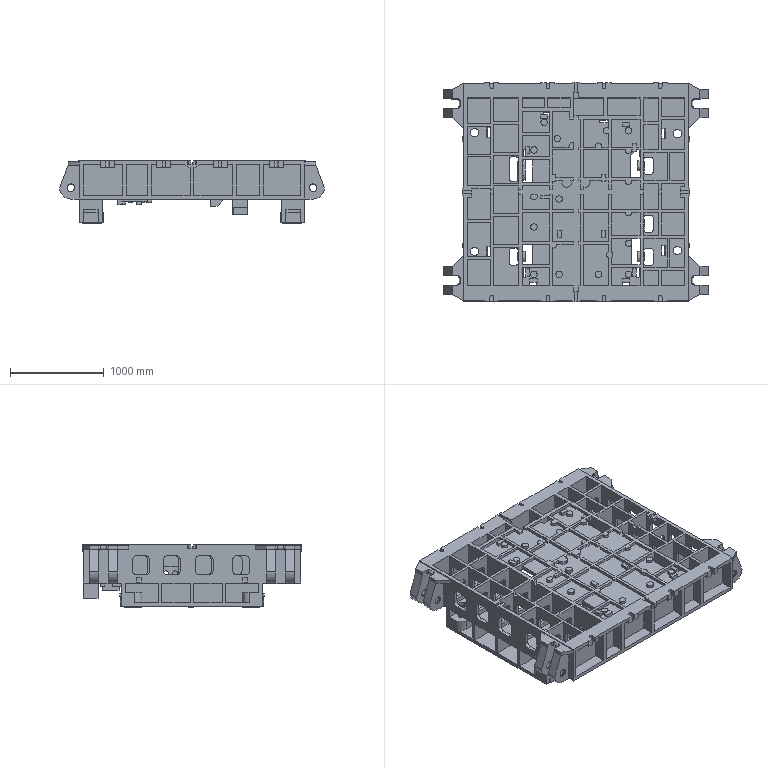Part | NX | features solid 2 | 1 solid | 1886 faces | box 2830 x 2350 x 670 mm | volume 725712954 mm3 | plane 1502 | cylinder 373 | torus 8 | cone 3 | commonest cylinder face diameters 80 x128 83 x48 30 x42 70 x42 50 x24 40 x20